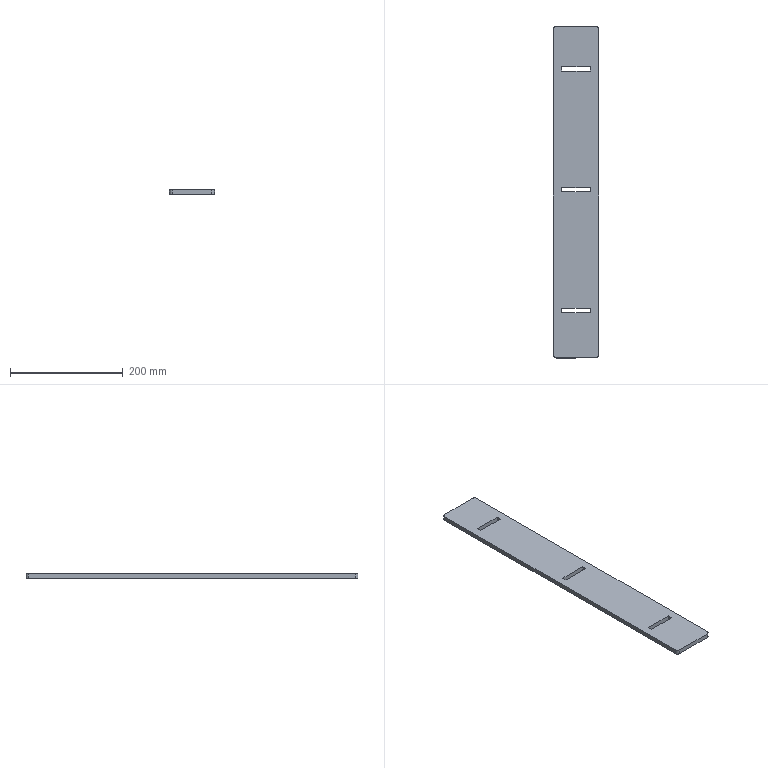Part | SolidWorks | features Fillet 1, FlatPattern 1, SMBaseFlange 1, SheetMetal 1 | 1 solid | 22 faces | box 80 x 590 x 8 mm | volume 367828 mm3 | plane 18 | cylinder 4 | commonest cylinder face diameters 10 x4
STEP:
#1=CARTESIAN_POINT('',(214.314,-80.,8.));
#2=VERTEX_POINT('',#1);
#3=CARTESIAN_POINT('',(284.314,-80.,8.));
#4=VERTEX_POINT('',#3);
#5=CARTESIAN_POINT('',(289.314,-80.,8.));
#6=DIRECTION('',(1.,0.,0.));
#7=VECTOR('',#6,1000.);
#8=LINE('',#5,#7);
#9=EDGE_CURVE('',#2,#4,#8,.T.);
#10=ORIENTED_EDGE('',*,*,#9,.T.);
#11=CARTESIAN_POINT('',(289.314,-75.,8.));
#12=VERTEX_POINT('',#11);
#13=CARTESIAN_POINT('',(284.314,-75.,8.));
#14=DIRECTION('',(0.,0.,1.));
#15=DIRECTION('',(1.,0.,0.));
#16=AXIS2_PLACEMENT_3D('',#13,#14,#15);
#17=CIRCLE('',#16,5.);
#18=EDGE_CURVE('',#4,#12,#17,.T.);
#19=ORIENTED_EDGE('',*,*,#18,.T.);
#20=CARTESIAN_POINT('',(289.314,505.,8.));
#21=VERTEX_POINT('',#20);
#22=CARTESIAN_POINT('',(289.314,-80.,8.));
#23=DIRECTION('',(0.,1.,0.));
#24=VECTOR('',#23,1000.);
#25=LINE('',#22,#24);
#26=EDGE_CURVE('',#12,#21,#25,.T.);
#27=ORIENTED_EDGE('',*,*,#26,.T.);
#28=CARTESIAN_POINT('',(284.314,510.,8.));
#29=VERTEX_POINT('',#28);
#30=CARTESIAN_POINT('',(284.314,505.,8.));
#31=DIRECTION('',(0.,0.,1.));
#32=DIRECTION('',(1.,0.,0.));
#33=AXIS2_PLACEMENT_3D('',#30,#31,#32);
#34=CIRCLE('',#33,5.);
#35=EDGE_CURVE('',#21,#29,#34,.T.);
#36=ORIENTED_EDGE('',*,*,#35,.T.);
#37=CARTESIAN_POINT('',(214.314,510.,8.));
#38=VERTEX_POINT('',#37);
#39=CARTESIAN_POINT('',(289.314,510.,8.));
#40=DIRECTION('',(-1.,0.,0.));
#41=VECTOR('',#40,1000.);
#42=LINE('',#39,#41);
#43=EDGE_CURVE('',#29,#38,#42,.T.);
#44=ORIENTED_EDGE('',*,*,#43,.T.);
#45=CARTESIAN_POINT('',(209.314,505.,8.));
#46=VERTEX_POINT('',#45);
#47=CARTESIAN_POINT('',(214.314,505.,8.));
#48=DIRECTION('',(0.,0.,1.));
#49=DIRECTION('',(1.,0.,0.));
#50=AXIS2_PLACEMENT_3D('',#47,#48,#49);
#51=CIRCLE('',#50,5.);
#52=EDGE_CURVE('',#38,#46,#51,.T.);
#53=ORIENTED_EDGE('',*,*,#52,.T.);
#54=CARTESIAN_POINT('',(209.314,-75.,8.));
#55=VERTEX_POINT('',#54);
#56=CARTESIAN_POINT('',(209.314,-80.,8.));
#57=DIRECTION('',(0.,-1.,0.));
#58=VECTOR('',#57,1000.);
#59=LINE('',#56,#58);
#60=EDGE_CURVE('',#46,#55,#59,.T.);
#61=ORIENTED_EDGE('',*,*,#60,.T.);
#62=CARTESIAN_POINT('',(214.314,-75.,8.));
#63=DIRECTION('',(0.,0.,1.));
#64=DIRECTION('',(1.,0.,0.));
#65=AXIS2_PLACEMENT_3D('',#62,#63,#64);
#66=CIRCLE('',#65,5.);
#67=EDGE_CURVE('',#55,#2,#66,.T.);
#68=ORIENTED_EDGE('',*,*,#67,.T.);
#69=EDGE_LOOP('',(#10,#19,#27,#36,#44,#53,#61,#68));
#70=FACE_OUTER_BOUND('',#69,.T.);
#71=CARTESIAN_POINT('',(274.314,223.,8.));
#72=VERTEX_POINT('',#71);
#73=CARTESIAN_POINT('',(224.314,223.,8.));
#74=VERTEX_POINT('',#73);
#75=CARTESIAN_POINT('',(274.314,223.,8.));
#76=DIRECTION('',(-1.,0.,0.));
#77=VECTOR('',#76,1000.);
#78=LINE('',#75,#77);
#79=EDGE_CURVE('',#72,#74,#78,.T.);
#80=ORIENTED_EDGE('',*,*,#79,.F.);
#81=CARTESIAN_POINT('',(274.314,215.,8.));
#82=VERTEX_POINT('',#81);
#83=CARTESIAN_POINT('',(274.314,223.,8.));
#84=DIRECTION('',(0.,1.,0.));
#85=VECTOR('',#84,1000.);
#86=LINE('',#83,#85);
#87=EDGE_CURVE('',#82,#72,#86,.T.);
#88=ORIENTED_EDGE('',*,*,#87,.F.);
#89=CARTESIAN_POINT('',(224.314,215.,8.));
#90=VERTEX_POINT('',#89);
#91=CARTESIAN_POINT('',(274.314,215.,8.));
#92=DIRECTION('',(1.,0.,0.));
#93=VECTOR('',#92,1000.);
#94=LINE('',#91,#93);
#95=EDGE_CURVE('',#90,#82,#94,.T.);
#96=ORIENTED_EDGE('',*,*,#95,.F.);
#97=CARTESIAN_POINT('',(224.314,223.,8.));
#98=DIRECTION('',(0.,-1.,0.));
#99=VECTOR('',#98,1000.);
#100=LINE('',#97,#99);
#101=EDGE_CURVE('',#74,#90,#100,.T.);
#102=ORIENTED_EDGE('',*,*,#101,.F.);
#103=EDGE_LOOP('',(#80,#88,#96,#102));
#104=FACE_BOUND('',#103,.T.);
#105=CARTESIAN_POINT('',(274.314,8.,8.));
#106=VERTEX_POINT('',#105);
#107=CARTESIAN_POINT('',(224.314,8.,8.));
#108=VERTEX_POINT('',#107);
#109=CARTESIAN_POINT('',(274.314,8.,8.));
#110=DIRECTION('',(-1.,0.,0.));
#111=VECTOR('',#110,1000.);
#112=LINE('',#109,#111);
#113=EDGE_CURVE('',#106,#108,#112,.T.);
#114=ORIENTED_EDGE('',*,*,#113,.F.);
#115=CARTESIAN_POINT('',(274.314,0.,8.));
#116=VERTEX_POINT('',#115);
#117=CARTESIAN_POINT('',(274.314,0.,8.));
#118=DIRECTION('',(0.,1.,0.));
#119=VECTOR('',#118,1000.);
#120=LINE('',#117,#119);
#121=EDGE_CURVE('',#116,#106,#120,.T.);
#122=ORIENTED_EDGE('',*,*,#121,.F.);
#123=CARTESIAN_POINT('',(224.314,0.,8.));
#124=VERTEX_POINT('',#123);
#125=CARTESIAN_POINT('',(274.314,0.,8.));
#126=DIRECTION('',(1.,0.,0.));
#127=VECTOR('',#126,1000.);
#128=LINE('',#125,#127);
#129=EDGE_CURVE('',#124,#116,#128,.T.);
#130=ORIENTED_EDGE('',*,*,#129,.F.);
#131=CARTESIAN_POINT('',(224.314,0.,8.));
#132=DIRECTION('',(0.,-1.,0.));
#133=VECTOR('',#132,1000.);
#134=LINE('',#131,#133);
#135=EDGE_CURVE('',#108,#124,#134,.T.);
#136=ORIENTED_EDGE('',*,*,#135,.F.);
#137=EDGE_LOOP('',(#114,#122,#130,#136));
#138=FACE_BOUND('',#137,.T.);
#139=CARTESIAN_POINT('',(224.314,430.,8.));
#140=VERTEX_POINT('',#139);
#141=CARTESIAN_POINT('',(274.314,430.,8.));
#142=VERTEX_POINT('',#141);
#143=CARTESIAN_POINT('',(224.314,430.,8.));
#144=DIRECTION('',(1.,0.,0.));
#145=VECTOR('',#144,1000.);
#146=LINE('',#143,#145);
#147=EDGE_CURVE('',#140,#142,#146,.T.);
#148=ORIENTED_EDGE('',*,*,#147,.F.);
#149=CARTESIAN_POINT('',(224.314,438.,8.));
#150=VERTEX_POINT('',#149);
#151=CARTESIAN_POINT('',(224.314,438.,8.));
#152=DIRECTION('',(0.,-1.,0.));
#153=VECTOR('',#152,1000.);
#154=LINE('',#151,#153);
#155=EDGE_CURVE('',#150,#140,#154,.T.);
#156=ORIENTED_EDGE('',*,*,#155,.F.);
#157=CARTESIAN_POINT('',(274.314,438.,8.));
#158=VERTEX_POINT('',#157);
#159=CARTESIAN_POINT('',(224.314,438.,8.));
#160=DIRECTION('',(-1.,0.,0.));
#161=VECTOR('',#160,1000.);
#162=LINE('',#159,#161);
#163=EDGE_CURVE('',#158,#150,#162,.T.);
#164=ORIENTED_EDGE('',*,*,#163,.F.);
#165=CARTESIAN_POINT('',(274.314,438.,8.));
#166=DIRECTION('',(0.,1.,0.));
#167=VECTOR('',#166,1000.);
#168=LINE('',#165,#167);
#169=EDGE_CURVE('',#142,#158,#168,.T.);
#170=ORIENTED_EDGE('',*,*,#169,.F.);
#171=EDGE_LOOP('',(#148,#156,#164,#170));
#172=FACE_BOUND('',#171,.T.);
#173=CARTESIAN_POINT('',(0.,0.,8.));
#174=DIRECTION('',(0.,0.,1.));
#175=DIRECTION('',(1.,0.,0.));
#176=AXIS2_PLACEMENT_3D('',#173,#174,#175);
#177=PLANE('',#176);
#178=ADVANCED_FACE('',(#70,#104,#138,#172),#177,.T.);
#179=CARTESIAN_POINT('',(274.314,0.,0.));
#180=VERTEX_POINT('',#179);
#181=CARTESIAN_POINT('',(274.314,8.,0.));
#182=VERTEX_POINT('',#181);
#183=CARTESIAN_POINT('',(274.314,0.,0.));
#184=DIRECTION('',(0.,1.,0.));
#185=VECTOR('',#184,1000.);
#186=LINE('',#183,#185);
#187=EDGE_CURVE('',#180,#182,#186,.T.);
#188=ORIENTED_EDGE('',*,*,#187,.T.);
#189=CARTESIAN_POINT('',(224.314,8.,0.));
#190=VERTEX_POINT('',#189);
#191=CARTESIAN_POINT('',(274.314,8.,0.));
#192=DIRECTION('',(-1.,0.,0.));
#193=VECTOR('',#192,1000.);
#194=LINE('',#191,#193);
#195=EDGE_CURVE('',#182,#190,#194,.T.);
#196=ORIENTED_EDGE('',*,*,#195,.T.);
#197=CARTESIAN_POINT('',(224.314,0.,0.));
#198=VERTEX_POINT('',#197);
#199=CARTESIAN_POINT('',(224.314,0.,0.));
#200=DIRECTION('',(0.,-1.,0.));
#201=VECTOR('',#200,1000.);
#202=LINE('',#199,#201);
#203=EDGE_CURVE('',#190,#198,#202,.T.);
#204=ORIENTED_EDGE('',*,*,#203,.T.);
#205=CARTESIAN_POINT('',(274.314,0.,0.));
#206=DIRECTION('',(1.,0.,0.));
#207=VECTOR('',#206,1000.);
#208=LINE('',#205,#207);
#209=EDGE_CURVE('',#198,#180,#208,.T.);
#210=ORIENTED_EDGE('',*,*,#209,.T.);
#211=EDGE_LOOP('',(#188,#196,#204,#210));
#212=FACE_BOUND('',#211,.T.);
#213=CARTESIAN_POINT('',(289.314,-75.,0.));
#214=VERTEX_POINT('',#213);
#215=CARTESIAN_POINT('',(289.314,505.,0.));
#216=VERTEX_POINT('',#215);
#217=CARTESIAN_POINT('',(289.314,-80.,0.));
#218=DIRECTION('',(0.,1.,0.));
#219=VECTOR('',#218,1000.);
#220=LINE('',#217,#219);
#221=EDGE_CURVE('',#214,#216,#220,.T.);
#222=ORIENTED_EDGE('',*,*,#221,.F.);
#223=CARTESIAN_POINT('',(284.314,-80.,0.));
#224=VERTEX_POINT('',#223);
#225=CARTESIAN_POINT('',(284.314,-75.,0.));
#226=DIRECTION('',(0.,0.,-1.));
#227=DIRECTION('',(1.,0.,0.));
#228=AXIS2_PLACEMENT_3D('',#225,#226,#227);
#229=CIRCLE('',#228,5.);
#230=EDGE_CURVE('',#214,#224,#229,.T.);
#231=ORIENTED_EDGE('',*,*,#230,.T.);
#232=CARTESIAN_POINT('',(214.314,-80.,0.));
#233=VERTEX_POINT('',#232);
#234=CARTESIAN_POINT('',(289.314,-80.,0.));
#235=DIRECTION('',(1.,0.,0.));
#236=VECTOR('',#235,1000.);
#237=LINE('',#234,#236);
#238=EDGE_CURVE('',#233,#224,#237,.T.);
#239=ORIENTED_EDGE('',*,*,#238,.F.);
#240=CARTESIAN_POINT('',(209.314,-75.,0.));
#241=VERTEX_POINT('',#240);
#242=CARTESIAN_POINT('',(214.314,-75.,0.));
#243=DIRECTION('',(0.,0.,-1.));
#244=DIRECTION('',(1.,0.,0.));
#245=AXIS2_PLACEMENT_3D('',#242,#243,#244);
#246=CIRCLE('',#245,5.);
#247=EDGE_CURVE('',#233,#241,#246,.T.);
#248=ORIENTED_EDGE('',*,*,#247,.T.);
#249=CARTESIAN_POINT('',(209.314,505.,0.));
#250=VERTEX_POINT('',#249);
#251=CARTESIAN_POINT('',(209.314,-80.,0.));
#252=DIRECTION('',(0.,-1.,0.));
#253=VECTOR('',#252,1000.);
#254=LINE('',#251,#253);
#255=EDGE_CURVE('',#250,#241,#254,.T.);
#256=ORIENTED_EDGE('',*,*,#255,.F.);
#257=CARTESIAN_POINT('',(214.314,510.,0.));
#258=VERTEX_POINT('',#257);
#259=CARTESIAN_POINT('',(214.314,505.,0.));
#260=DIRECTION('',(0.,0.,-1.));
#261=DIRECTION('',(1.,0.,0.));
#262=AXIS2_PLACEMENT_3D('',#259,#260,#261);
#263=CIRCLE('',#262,5.);
#264=EDGE_CURVE('',#250,#258,#263,.T.);
#265=ORIENTED_EDGE('',*,*,#264,.T.);
#266=CARTESIAN_POINT('',(284.314,510.,0.));
#267=VERTEX_POINT('',#266);
#268=CARTESIAN_POINT('',(289.314,510.,0.));
#269=DIRECTION('',(-1.,0.,0.));
#270=VECTOR('',#269,1000.);
#271=LINE('',#268,#270);
#272=EDGE_CURVE('',#267,#258,#271,.T.);
#273=ORIENTED_EDGE('',*,*,#272,.F.);
#274=CARTESIAN_POINT('',(284.314,505.,0.));
#275=DIRECTION('',(0.,0.,-1.));
#276=DIRECTION('',(1.,0.,0.));
#277=AXIS2_PLACEMENT_3D('',#274,#275,#276);
#278=CIRCLE('',#277,5.);
#279=EDGE_CURVE('',#267,#216,#278,.T.);
#280=ORIENTED_EDGE('',*,*,#279,.T.);
#281=EDGE_LOOP('',(#222,#231,#239,#248,#256,#265,#273,#280));
#282=FACE_OUTER_BOUND('',#281,.T.);
#283=CARTESIAN_POINT('',(274.314,215.,0.));
#284=VERTEX_POINT('',#283);
#285=CARTESIAN_POINT('',(274.314,223.,0.));
#286=VERTEX_POINT('',#285);
#287=CARTESIAN_POINT('',(274.314,223.,0.));
#288=DIRECTION('',(0.,1.,0.));
#289=VECTOR('',#288,1000.);
#290=LINE('',#287,#289);
#291=EDGE_CURVE('',#284,#286,#290,.T.);
#292=ORIENTED_EDGE('',*,*,#291,.T.);
#293=CARTESIAN_POINT('',(224.314,223.,0.));
#294=VERTEX_POINT('',#293);
#295=CARTESIAN_POINT('',(274.314,223.,0.));
#296=DIRECTION('',(-1.,0.,0.));
#297=VECTOR('',#296,1000.);
#298=LINE('',#295,#297);
#299=EDGE_CURVE('',#286,#294,#298,.T.);
#300=ORIENTED_EDGE('',*,*,#299,.T.);
#301=CARTESIAN_POINT('',(224.314,215.,0.));
#302=VERTEX_POINT('',#301);
#303=CARTESIAN_POINT('',(224.314,223.,0.));
#304=DIRECTION('',(0.,-1.,0.));
#305=VECTOR('',#304,1000.);
#306=LINE('',#303,#305);
#307=EDGE_CURVE('',#294,#302,#306,.T.);
#308=ORIENTED_EDGE('',*,*,#307,.T.);
#309=CARTESIAN_POINT('',(274.314,215.,0.));
#310=DIRECTION('',(1.,0.,0.));
#311=VECTOR('',#310,1000.);
#312=LINE('',#309,#311);
#313=EDGE_CURVE('',#302,#284,#312,.T.);
#314=ORIENTED_EDGE('',*,*,#313,.T.);
#315=EDGE_LOOP('',(#292,#300,#308,#314));
#316=FACE_BOUND('',#315,.T.);
#317=CARTESIAN_POINT('',(224.314,438.,0.));
#318=VERTEX_POINT('',#317);
#319=CARTESIAN_POINT('',(224.314,430.,0.));
#320=VERTEX_POINT('',#319);
#321=CARTESIAN_POINT('',(224.314,438.,0.));
#322=DIRECTION('',(0.,-1.,0.));
#323=VECTOR('',#322,1000.);
#324=LINE('',#321,#323);
#325=EDGE_CURVE('',#318,#320,#324,.T.);
#326=ORIENTED_EDGE('',*,*,#325,.T.);
#327=CARTESIAN_POINT('',(274.314,430.,0.));
#328=VERTEX_POINT('',#327);
#329=CARTESIAN_POINT('',(224.314,430.,0.));
#330=DIRECTION('',(1.,0.,0.));
#331=VECTOR('',#330,1000.);
#332=LINE('',#329,#331);
#333=EDGE_CURVE('',#320,#328,#332,.T.);
#334=ORIENTED_EDGE('',*,*,#333,.T.);
#335=CARTESIAN_POINT('',(274.314,438.,0.));
#336=VERTEX_POINT('',#335);
#337=CARTESIAN_POINT('',(274.314,438.,0.));
#338=DIRECTION('',(0.,1.,0.));
#339=VECTOR('',#338,1000.);
#340=LINE('',#337,#339);
#341=EDGE_CURVE('',#328,#336,#340,.T.);
#342=ORIENTED_EDGE('',*,*,#341,.T.);
#343=CARTESIAN_POINT('',(224.314,438.,0.));
#344=DIRECTION('',(-1.,0.,0.));
#345=VECTOR('',#344,1000.);
#346=LINE('',#343,#345);
#347=EDGE_CURVE('',#336,#318,#346,.T.);
#348=ORIENTED_EDGE('',*,*,#347,.T.);
#349=EDGE_LOOP('',(#326,#334,#342,#348));
#350=FACE_BOUND('',#349,.T.);
#351=CARTESIAN_POINT('',(0.,0.,0.));
#352=DIRECTION('',(0.,0.,1.));
#353=DIRECTION('',(1.,0.,0.));
#354=AXIS2_PLACEMENT_3D('',#351,#352,#353);
#355=PLANE('',#354);
#356=ADVANCED_FACE('',(#212,#282,#316,#350),#355,.F.);
#357=ORIENTED_EDGE('',*,*,#26,.F.);
#358=CARTESIAN_POINT('',(289.314,-75.,8.));
#359=DIRECTION('',(0.,0.,-1.));
#360=VECTOR('',#359,1000.);
#361=LINE('',#358,#360);
#362=EDGE_CURVE('',#12,#214,#361,.T.);
#363=ORIENTED_EDGE('',*,*,#362,.T.);
#364=ORIENTED_EDGE('',*,*,#221,.T.);
#365=CARTESIAN_POINT('',(289.314,505.,8.));
#366=DIRECTION('',(0.,0.,1.));
#367=VECTOR('',#366,1000.);
#368=LINE('',#365,#367);
#369=EDGE_CURVE('',#216,#21,#368,.T.);
#370=ORIENTED_EDGE('',*,*,#369,.T.);
#371=EDGE_LOOP('',(#357,#363,#364,#370));
#372=FACE_OUTER_BOUND('',#371,.T.);
#373=CARTESIAN_POINT('',(289.314,-80.,8.));
#374=DIRECTION('',(-1.,0.,0.));
#375=DIRECTION('',(0.,0.,1.));
#376=AXIS2_PLACEMENT_3D('',#373,#374,#375);
#377=PLANE('',#376);
#378=ADVANCED_FACE('',(#372),#377,.F.);
#379=ORIENTED_EDGE('',*,*,#43,.F.);
#380=CARTESIAN_POINT('',(284.314,510.,8.));
#381=DIRECTION('',(0.,0.,-1.));
#382=VECTOR('',#381,1000.);
#383=LINE('',#380,#382);
#384=EDGE_CURVE('',#29,#267,#383,.T.);
#385=ORIENTED_EDGE('',*,*,#384,.T.);
#386=ORIENTED_EDGE('',*,*,#272,.T.);
#387=CARTESIAN_POINT('',(214.314,510.,8.));
#388=DIRECTION('',(0.,0.,1.));
#389=VECTOR('',#388,1000.);
#390=LINE('',#387,#389);
#391=EDGE_CURVE('',#258,#38,#390,.T.);
#392=ORIENTED_EDGE('',*,*,#391,.T.);
#393=EDGE_LOOP('',(#379,#385,#386,#392));
#394=FACE_OUTER_BOUND('',#393,.T.);
#395=CARTESIAN_POINT('',(289.314,510.,8.));
#396=DIRECTION('',(0.,-1.,0.));
#397=DIRECTION('',(0.,0.,-1.));
#398=AXIS2_PLACEMENT_3D('',#395,#396,#397);
#399=PLANE('',#398);
#400=ADVANCED_FACE('',(#394),#399,.F.);
#401=ORIENTED_EDGE('',*,*,#255,.T.);
#402=CARTESIAN_POINT('',(209.314,-75.,8.));
#403=DIRECTION('',(0.,0.,1.));
#404=VECTOR('',#403,1000.);
#405=LINE('',#402,#404);
#406=EDGE_CURVE('',#241,#55,#405,.T.);
#407=ORIENTED_EDGE('',*,*,#406,.T.);
#408=ORIENTED_EDGE('',*,*,#60,.F.);
#409=CARTESIAN_POINT('',(209.314,505.,8.));
#410=DIRECTION('',(0.,0.,-1.));
#411=VECTOR('',#410,1000.);
#412=LINE('',#409,#411);
#413=EDGE_CURVE('',#46,#250,#412,.T.);
#414=ORIENTED_EDGE('',*,*,#413,.T.);
#415=EDGE_LOOP('',(#401,#407,#408,#414));
#416=FACE_OUTER_BOUND('',#415,.T.);
#417=CARTESIAN_POINT('',(209.314,-80.,8.));
#418=DIRECTION('',(1.,0.,0.));
#419=DIRECTION('',(0.,0.,-1.));
#420=AXIS2_PLACEMENT_3D('',#417,#418,#419);
#421=PLANE('',#420);
#422=ADVANCED_FACE('',(#416),#421,.F.);
#423=ORIENTED_EDGE('',*,*,#238,.T.);
#424=CARTESIAN_POINT('',(284.314,-80.,8.));
#425=DIRECTION('',(0.,0.,1.));
#426=VECTOR('',#425,1000.);
#427=LINE('',#424,#426);
#428=EDGE_CURVE('',#224,#4,#427,.T.);
#429=ORIENTED_EDGE('',*,*,#428,.T.);
#430=ORIENTED_EDGE('',*,*,#9,.F.);
#431=CARTESIAN_POINT('',(214.314,-80.,8.));
#432=DIRECTION('',(0.,0.,-1.));
#433=VECTOR('',#432,1000.);
#434=LINE('',#431,#433);
#435=EDGE_CURVE('',#2,#233,#434,.T.);
#436=ORIENTED_EDGE('',*,*,#435,.T.);
#437=EDGE_LOOP('',(#423,#429,#430,#436));
#438=FACE_OUTER_BOUND('',#437,.T.);
#439=CARTESIAN_POINT('',(289.314,-80.,8.));
#440=DIRECTION('',(0.,1.,0.));
#441=DIRECTION('',(-1.,0.,0.));
#442=AXIS2_PLACEMENT_3D('',#439,#440,#441);
#443=PLANE('',#442);
#444=ADVANCED_FACE('',(#438),#443,.F.);
#445=ORIENTED_EDGE('',*,*,#291,.F.);
#446=CARTESIAN_POINT('',(274.314,215.,8.));
#447=DIRECTION('',(0.,0.,-1.));
#448=VECTOR('',#447,1000.);
#449=LINE('',#446,#448);
#450=EDGE_CURVE('',#82,#284,#449,.T.);
#451=ORIENTED_EDGE('',*,*,#450,.F.);
#452=ORIENTED_EDGE('',*,*,#87,.T.);
#453=CARTESIAN_POINT('',(274.314,223.,8.));
#454=DIRECTION('',(0.,0.,-1.));
#455=VECTOR('',#454,1000.);
#456=LINE('',#453,#455);
#457=EDGE_CURVE('',#72,#286,#456,.T.);
#458=ORIENTED_EDGE('',*,*,#457,.T.);
#459=EDGE_LOOP('',(#445,#451,#452,#458));
#460=FACE_OUTER_BOUND('',#459,.T.);
#461=CARTESIAN_POINT('',(274.314,223.,8.));
#462=DIRECTION('',(-1.,0.,0.));
#463=DIRECTION('',(0.,0.,1.));
#464=AXIS2_PLACEMENT_3D('',#461,#462,#463);
#465=PLANE('',#464);
#466=ADVANCED_FACE('',(#460),#465,.T.);
#467=ORIENTED_EDGE('',*,*,#299,.F.);
#468=ORIENTED_EDGE('',*,*,#457,.F.);
#469=ORIENTED_EDGE('',*,*,#79,.T.);
#470=CARTESIAN_POINT('',(224.314,223.,8.));
#471=DIRECTION('',(0.,0.,-1.));
#472=VECTOR('',#471,1000.);
#473=LINE('',#470,#472);
#474=EDGE_CURVE('',#74,#294,#473,.T.);
#475=ORIENTED_EDGE('',*,*,#474,.T.);
#476=EDGE_LOOP('',(#467,#468,#469,#475));
#477=FACE_OUTER_BOUND('',#476,.T.);
#478=CARTESIAN_POINT('',(274.314,223.,8.));
#479=DIRECTION('',(0.,-1.,0.));
#480=DIRECTION('',(0.,0.,-1.));
#481=AXIS2_PLACEMENT_3D('',#478,#479,#480);
#482=PLANE('',#481);
#483=ADVANCED_FACE('',(#477),#482,.T.);
#484=ORIENTED_EDGE('',*,*,#307,.F.);
#485=ORIENTED_EDGE('',*,*,#474,.F.);
#486=ORIENTED_EDGE('',*,*,#101,.T.);
#487=CARTESIAN_POINT('',(224.314,215.,8.));
#488=DIRECTION('',(0.,0.,-1.));
#489=VECTOR('',#488,1000.);
#490=LINE('',#487,#489);
#491=EDGE_CURVE('',#90,#302,#490,.T.);
#492=ORIENTED_EDGE('',*,*,#491,.T.);
#493=EDGE_LOOP('',(#484,#485,#486,#492));
#494=FACE_OUTER_BOUND('',#493,.T.);
#495=CARTESIAN_POINT('',(224.314,223.,8.));
#496=DIRECTION('',(1.,0.,0.));
#497=DIRECTION('',(0.,0.,-1.));
#498=AXIS2_PLACEMENT_3D('',#495,#496,#497);
#499=PLANE('',#498);
#500=ADVANCED_FACE('',(#494),#499,.T.);
#501=ORIENTED_EDGE('',*,*,#313,.F.);
#502=ORIENTED_EDGE('',*,*,#491,.F.);
#503=ORIENTED_EDGE('',*,*,#95,.T.);
#504=ORIENTED_EDGE('',*,*,#450,.T.);
#505=EDGE_LOOP('',(#501,#502,#503,#504));
#506=FACE_OUTER_BOUND('',#505,.T.);
#507=CARTESIAN_POINT('',(274.314,215.,8.));
#508=DIRECTION('',(0.,1.,0.));
#509=DIRECTION('',(0.,0.,1.));
#510=AXIS2_PLACEMENT_3D('',#507,#508,#509);
#511=PLANE('',#510);
#512=ADVANCED_FACE('',(#506),#511,.T.);
#513=ORIENTED_EDGE('',*,*,#187,.F.);
#514=CARTESIAN_POINT('',(274.314,0.,8.));
#515=DIRECTION('',(0.,0.,-1.));
#516=VECTOR('',#515,1000.);
#517=LINE('',#514,#516);
#518=EDGE_CURVE('',#116,#180,#517,.T.);
#519=ORIENTED_EDGE('',*,*,#518,.F.);
#520=ORIENTED_EDGE('',*,*,#121,.T.);
#521=CARTESIAN_POINT('',(274.314,8.,8.));
#522=DIRECTION('',(0.,0.,-1.));
#523=VECTOR('',#522,1000.);
#524=LINE('',#521,#523);
#525=EDGE_CURVE('',#106,#182,#524,.T.);
#526=ORIENTED_EDGE('',*,*,#525,.T.);
#527=EDGE_LOOP('',(#513,#519,#520,#526));
#528=FACE_OUTER_BOUND('',#527,.T.);
#529=CARTESIAN_POINT('',(274.314,0.,8.));
#530=DIRECTION('',(-1.,0.,0.));
#531=DIRECTION('',(0.,0.,1.));
#532=AXIS2_PLACEMENT_3D('',#529,#530,#531);
#533=PLANE('',#532);
#534=ADVANCED_FACE('',(#528),#533,.T.);
#535=ORIENTED_EDGE('',*,*,#195,.F.);
#536=ORIENTED_EDGE('',*,*,#525,.F.);
#537=ORIENTED_EDGE('',*,*,#113,.T.);
#538=CARTESIAN_POINT('',(224.314,8.,8.));
#539=DIRECTION('',(0.,0.,-1.));
#540=VECTOR('',#539,1000.);
#541=LINE('',#538,#540);
#542=EDGE_CURVE('',#108,#190,#541,.T.);
#543=ORIENTED_EDGE('',*,*,#542,.T.);
#544=EDGE_LOOP('',(#535,#536,#537,#543));
#545=FACE_OUTER_BOUND('',#544,.T.);
#546=CARTESIAN_POINT('',(274.314,8.,8.));
#547=DIRECTION('',(0.,-1.,0.));
#548=DIRECTION('',(0.,0.,-1.));
#549=AXIS2_PLACEMENT_3D('',#546,#547,#548);
#550=PLANE('',#549);
#551=ADVANCED_FACE('',(#545),#550,.T.);
#552=ORIENTED_EDGE('',*,*,#203,.F.);
#553=ORIENTED_EDGE('',*,*,#542,.F.);
#554=ORIENTED_EDGE('',*,*,#135,.T.);
#555=CARTESIAN_POINT('',(224.314,0.,8.));
#556=DIRECTION('',(0.,0.,-1.));
#557=VECTOR('',#556,1000.);
#558=LINE('',#555,#557);
#559=EDGE_CURVE('',#124,#198,#558,.T.);
#560=ORIENTED_EDGE('',*,*,#559,.T.);
#561=EDGE_LOOP('',(#552,#553,#554,#560));
#562=FACE_OUTER_BOUND('',#561,.T.);
#563=CARTESIAN_POINT('',(224.314,0.,8.));
#564=DIRECTION('',(1.,0.,0.));
#565=DIRECTION('',(0.,0.,-1.));
#566=AXIS2_PLACEMENT_3D('',#563,#564,#565);
#567=PLANE('',#566);
#568=ADVANCED_FACE('',(#562),#567,.T.);
#569=ORIENTED_EDGE('',*,*,#209,.F.);
#570=ORIENTED_EDGE('',*,*,#559,.F.);
#571=ORIENTED_EDGE('',*,*,#129,.T.);
#572=ORIENTED_EDGE('',*,*,#518,.T.);
#573=EDGE_LOOP('',(#569,#570,#571,#572));
#574=FACE_OUTER_BOUND('',#573,.T.);
#575=CARTESIAN_POINT('',(274.314,0.,8.));
#576=DIRECTION('',(0.,1.,0.));
#577=DIRECTION('',(0.,0.,1.));
#578=AXIS2_PLACEMENT_3D('',#575,#576,#577);
#579=PLANE('',#578);
#580=ADVANCED_FACE('',(#574),#579,.T.);
#581=ORIENTED_EDGE('',*,*,#325,.F.);
#582=CARTESIAN_POINT('',(224.314,438.,8.));
#583=DIRECTION('',(0.,0.,-1.));
#584=VECTOR('',#583,1000.);
#585=LINE('',#582,#584);
#586=EDGE_CURVE('',#150,#318,#585,.T.);
#587=ORIENTED_EDGE('',*,*,#586,.F.);
#588=ORIENTED_EDGE('',*,*,#155,.T.);
#589=CARTESIAN_POINT('',(224.314,430.,8.));
#590=DIRECTION('',(0.,0.,-1.));
#591=VECTOR('',#590,1000.);
#592=LINE('',#589,#591);
#593=EDGE_CURVE('',#140,#320,#592,.T.);
#594=ORIENTED_EDGE('',*,*,#593,.T.);
#595=EDGE_LOOP('',(#581,#587,#588,#594));
#596=FACE_OUTER_BOUND('',#595,.T.);
#597=CARTESIAN_POINT('',(224.314,438.,8.));
#598=DIRECTION('',(1.,0.,0.));
#599=DIRECTION('',(0.,0.,-1.));
#600=AXIS2_PLACEMENT_3D('',#597,#598,#599);
#601=PLANE('',#600);
#602=ADVANCED_FACE('',(#596),#601,.T.);
#603=ORIENTED_EDGE('',*,*,#333,.F.);
#604=ORIENTED_EDGE('',*,*,#593,.F.);
#605=ORIENTED_EDGE('',*,*,#147,.T.);
#606=CARTESIAN_POINT('',(274.314,430.,8.));
#607=DIRECTION('',(0.,0.,-1.));
#608=VECTOR('',#607,1000.);
#609=LINE('',#606,#608);
#610=EDGE_CURVE('',#142,#328,#609,.T.);
#611=ORIENTED_EDGE('',*,*,#610,.T.);
#612=EDGE_LOOP('',(#603,#604,#605,#611));
#613=FACE_OUTER_BOUND('',#612,.T.);
#614=CARTESIAN_POINT('',(224.314,430.,8.));
#615=DIRECTION('',(0.,1.,0.));
#616=DIRECTION('',(0.,0.,1.));
#617=AXIS2_PLACEMENT_3D('',#614,#615,#616);
#618=PLANE('',#617);
#619=ADVANCED_FACE('',(#613),#618,.T.);
#620=ORIENTED_EDGE('',*,*,#341,.F.);
#621=ORIENTED_EDGE('',*,*,#610,.F.);
#622=ORIENTED_EDGE('',*,*,#169,.T.);
#623=CARTESIAN_POINT('',(274.314,438.,8.));
#624=DIRECTION('',(0.,0.,-1.));
#625=VECTOR('',#624,1000.);
#626=LINE('',#623,#625);
#627=EDGE_CURVE('',#158,#336,#626,.T.);
#628=ORIENTED_EDGE('',*,*,#627,.T.);
#629=EDGE_LOOP('',(#620,#621,#622,#628));
#630=FACE_OUTER_BOUND('',#629,.T.);
#631=CARTESIAN_POINT('',(274.314,438.,8.));
#632=DIRECTION('',(-1.,0.,0.));
#633=DIRECTION('',(0.,0.,1.));
#634=AXIS2_PLACEMENT_3D('',#631,#632,#633);
#635=PLANE('',#634);
#636=ADVANCED_FACE('',(#630),#635,.T.);
#637=ORIENTED_EDGE('',*,*,#347,.F.);
#638=ORIENTED_EDGE('',*,*,#627,.F.);
#639=ORIENTED_EDGE('',*,*,#163,.T.);
#640=ORIENTED_EDGE('',*,*,#586,.T.);
#641=EDGE_LOOP('',(#637,#638,#639,#640));
#642=FACE_OUTER_BOUND('',#641,.T.);
#643=CARTESIAN_POINT('',(224.314,438.,8.));
#644=DIRECTION('',(0.,-1.,0.));
#645=DIRECTION('',(0.,0.,-1.));
#646=AXIS2_PLACEMENT_3D('',#643,#644,#645);
#647=PLANE('',#646);
#648=ADVANCED_FACE('',(#642),#647,.T.);
#649=ORIENTED_EDGE('',*,*,#18,.F.);
#650=ORIENTED_EDGE('',*,*,#428,.F.);
#651=ORIENTED_EDGE('',*,*,#230,.F.);
#652=ORIENTED_EDGE('',*,*,#362,.F.);
#653=EDGE_LOOP('',(#649,#650,#651,#652));
#654=FACE_OUTER_BOUND('',#653,.T.);
#655=CARTESIAN_POINT('',(284.314,-75.,8.));
#656=DIRECTION('',(0.,0.,-1.));
#657=DIRECTION('',(-1.,0.,0.));
#658=AXIS2_PLACEMENT_3D('',#655,#656,#657);
#659=CYLINDRICAL_SURFACE('',#658,5.);
#660=ADVANCED_FACE('',(#654),#659,.T.);
#661=ORIENTED_EDGE('',*,*,#67,.F.);
#662=ORIENTED_EDGE('',*,*,#406,.F.);
#663=ORIENTED_EDGE('',*,*,#247,.F.);
#664=ORIENTED_EDGE('',*,*,#435,.F.);
#665=EDGE_LOOP('',(#661,#662,#663,#664));
#666=FACE_OUTER_BOUND('',#665,.T.);
#667=CARTESIAN_POINT('',(214.314,-75.,8.));
#668=DIRECTION('',(0.,0.,-1.));
#669=DIRECTION('',(-1.,0.,0.));
#670=AXIS2_PLACEMENT_3D('',#667,#668,#669);
#671=CYLINDRICAL_SURFACE('',#670,5.);
#672=ADVANCED_FACE('',(#666),#671,.T.);
#673=ORIENTED_EDGE('',*,*,#35,.F.);
#674=ORIENTED_EDGE('',*,*,#369,.F.);
#675=ORIENTED_EDGE('',*,*,#279,.F.);
#676=ORIENTED_EDGE('',*,*,#384,.F.);
#677=EDGE_LOOP('',(#673,#674,#675,#676));
#678=FACE_OUTER_BOUND('',#677,.T.);
#679=CARTESIAN_POINT('',(284.314,505.,8.));
#680=DIRECTION('',(0.,0.,-1.));
#681=DIRECTION('',(-1.,0.,0.));
#682=AXIS2_PLACEMENT_3D('',#679,#680,#681);
#683=CYLINDRICAL_SURFACE('',#682,5.);
#684=ADVANCED_FACE('',(#678),#683,.T.);
#685=ORIENTED_EDGE('',*,*,#52,.F.);
#686=ORIENTED_EDGE('',*,*,#391,.F.);
#687=ORIENTED_EDGE('',*,*,#264,.F.);
#688=ORIENTED_EDGE('',*,*,#413,.F.);
#689=EDGE_LOOP('',(#685,#686,#687,#688));
#690=FACE_OUTER_BOUND('',#689,.T.);
#691=CARTESIAN_POINT('',(214.314,505.,8.));
#692=DIRECTION('',(0.,0.,-1.));
#693=DIRECTION('',(-1.,0.,0.));
#694=AXIS2_PLACEMENT_3D('',#691,#692,#693);
#695=CYLINDRICAL_SURFACE('',#694,5.);
#696=ADVANCED_FACE('',(#690),#695,.T.);
#697=CLOSED_SHELL('',(#178,#356,#378,#400,#422,#444,#466,#483,#500,#512,#534,#551,#568,#580,#602,#619,#636,#648,#660,#672,#684,#696));
#698=MANIFOLD_SOLID_BREP('',#697);
#699=CARTESIAN_POINT('',(0.,0.,0.));
#700=DIRECTION('',(0.,0.,1.));
#701=DIRECTION('',(1.,0.,0.));
#702=AXIS2_PLACEMENT_3D('',#699,#700,#701);
#703=(LENGTH_UNIT()NAMED_UNIT(*)SI_UNIT(.MILLI.,.METRE.));
#704=UNCERTAINTY_MEASURE_WITH_UNIT(LENGTH_MEASURE(0.00001),#703,'','');
#705=(NAMED_UNIT(*)PLANE_ANGLE_UNIT()SI_UNIT($,.RADIAN.));
#706=(NAMED_UNIT(*)SI_UNIT($,.STERADIAN.)SOLID_ANGLE_UNIT());
#707=(GEOMETRIC_REPRESENTATION_CONTEXT(3)GLOBAL_UNCERTAINTY_ASSIGNED_CONTEXT((#704))GLOBAL_UNIT_ASSIGNED_CONTEXT((#703,#705,#706))REPRESENTATION_CONTEXT('',''));
#708=ADVANCED_BREP_SHAPE_REPRESENTATION('',(#698,#702),#707);